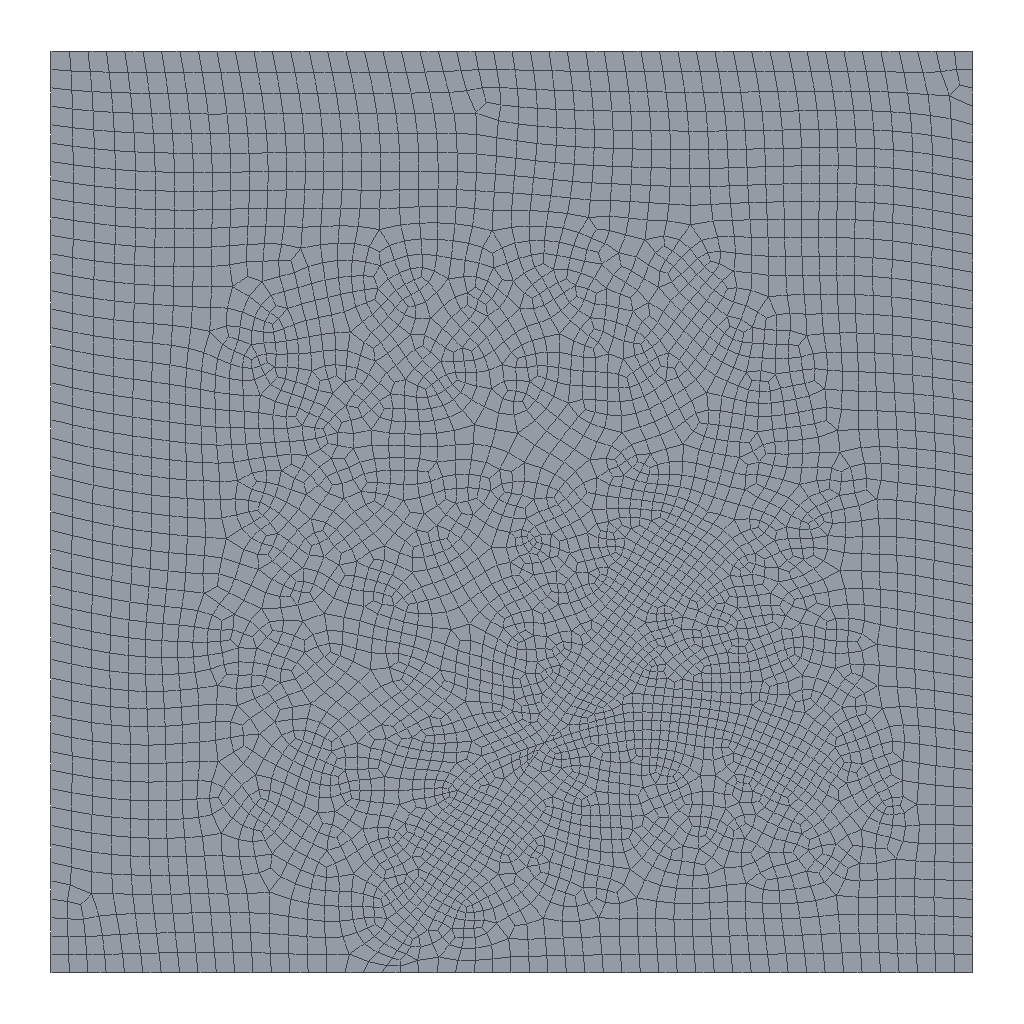Simulation study | abaqus
Set-up summary:
category,name,step,type,value,unit,region
solver,abaqus
solver,version,,,Abaqus/Standard 2020
units,not stated in the deck,,not stated
analysis,deck,,geostatic,geostatic
load_step,Step-1,Step-1,geostatic
load_step,Step-2,Step-2,soils
load_step,requested,,,2
mesh,nodes,,,4728
mesh,elements,,,4528
element_type,CPE4RP,,plane,4428
element_type,COH2D4P,,cohesive,100
load,load commands in deck,,count,1
bc,support commands in deck,,count,6
material,BASE,,in results
material,MATERIAL-2,,in results
check,setup vs results,,match,"per instance, exact: element labels, types and connectivity; labels of the nodes the elements use; coordinates of those nodes at SINGLE_PRECISION in 1 of 1 instance(s)"
Abaqus input file, long lists of numbers shortened:
*Heading
** Job name: Job-1 Model name: Model-1
** Generated by: Abaqus/CAE 2020
*Preprint, echo=NO, model=NO, history=NO, contact=NO
**
** PARTS
**
*Part, name=Part-1
*Node
      1,         100.,           0.
      2,           0.,           0.
** (4726 more lines like these left out)
*Element, type=CPE4RP
   1,    1,   10, 3981,  300
   2,  347,  394,  298,  299
** (4426 more lines like these left out)
*Element, type=COH2D4P
4429,    7,  187, 4530,    7,    7, 4592
4430,  187,  186, 4531, 4530, 4592, 4593
** (98 more lines like these left out)
*Nset, nset=Set-19
    1,    2,    3,    4,    5,    6,    7,    8,    9,   10,   11,   12,   13,   14,   15,   16
   17,   18,   19,   20,   21,   22,   23,   24,   25,   26,   27,   28,   29,   30,   31,   32
** (288 more lines like these left out)
*Elset, elset=Set-19, generate
    1,  4428,     1
*Elset, elset=CohesiveSeam-5-Elements, generate
 4429,  4490,     1
*Nset, nset=CohesiveSeam-5-TopNodes
    4,    5,    7,  125,  126,  127,  128,  129,  130,  131,  132,  133,  134,  135,  136,  137
  138,  139,  140,  141,  142,  143,  144,  145,  146,  147,  148,  149,  150,  151,  152,  153
** (2 more lines like these left out)
*Nset, nset=CohesiveSeam-5-BottomNodes
    7,  158,  159,  160,  161,  162,  163,  164,  165,  166,  167,  168,  169,  170,  171,  172
  173,  174,  175,  176,  177,  178,  179,  180,  181,  182,  183,  184,  185,  186,  187, 4561
** (2 more lines like these left out)
*Nset, nset=CohesiveSeam-5-MidNodes
    7, 4592, 4593, 4594, 4595, 4596, 4597, 4598, 4599, 4600, 4601, 4602, 4603, 4604, 4605, 4606
 4607, 4608, 4609, 4610, 4611, 4612, 4613, 4614, 4615, 4616, 4617, 4618, 4619, 4620, 4621, 4622
** (2 more lines like these left out)
*Elset, elset=CohesiveSeam-6-Elements, generate
 4491,  4528,     1
*Nset, nset=CohesiveSeam-6-TopNodes
    5,    6,    8,  155,  156,  157, 4659, 4660, 4661, 4662, 4663, 4664, 4665, 4666, 4667, 4668
 4669, 4670, 4671, 4672, 4673, 4674, 4675, 4676, 4677, 4678, 4679, 4680, 4681, 4682, 4683, 4684
** (1 more lines like these left out)
*Nset, nset=CohesiveSeam-6-BottomNodes
    6,    8,  188,  189,  190,  191,  192,  193,  194,  195,  196,  197,  198,  199,  200,  201
  202,  203,  204,  205,  206,  207,  208,  209,  210,  211,  212,  213,  214,  215,  216,  217
** (1 more lines like these left out)
*Nset, nset=CohesiveSeam-6-MidNodes
    6,    8, 4622, 4693, 4694, 4695, 4696, 4697, 4698, 4699, 4700, 4701, 4702, 4703, 4704, 4705
 4706, 4707, 4708, 4709, 4710, 4711, 4712, 4713, 4714, 4715, 4716, 4717, 4718, 4719, 4720, 4721
** (1 more lines like these left out)
*Nset, nset=inject
 4653,
*Elset, elset=initial-crack, generate
 4482,  4490,     1
*Nset, nset=plug1
 4621,
*Nset, nset=plug2
 4695,
*Elset, elset=__PickedSurf9_S1, internal
 1814, 1837, 1840, 1841, 1929, 1940, 2998, 3040, 3042, 3046, 3157, 4231, 4460, 4461, 4462, 4463
 4464, 4465, 4466, 4467, 4468, 4469, 4470, 4471, 4472, 4473, 4474, 4475, 4476, 4477, 4478, 4479
** (3 more lines like these left out)
*Elset, elset=__PickedSurf9_S4, internal
  359,  417,  449,  555, 1816, 1821, 1823, 1842, 2881, 3016, 3017, 3043, 3048, 3049, 3050, 3053
 3057, 3058, 3059, 3154
*Elset, elset=__PickedSurf9_S2, internal
  360,  416,  448,  484,  520,  554, 3037, 3039, 3045, 3055, 3060, 3125, 3131, 3144, 4232
*Elset, elset=__PickedSurf9_S3, internal
  362, 1791, 1825, 1839, 1878, 1892, 1893, 1894, 1902, 1928, 2914, 2937, 3038, 3044, 3047, 3051
 3052, 3056, 3141, 3149, 3158
*Surface, type=ELEMENT, name=_PickedSurf9, internal
__PickedSurf9_S1, S1
__PickedSurf9_S4, S4
__PickedSurf9_S2, S2
__PickedSurf9_S3, S3
*Elset, elset=__PickedSurf16_S1, internal, generate
 4460,  4490,     1
*Surface, type=ELEMENT, name=_PickedSurf16, internal
__PickedSurf16_S1, S1
*Elset, elset=__PickedSurf23_S4, internal
  359,  417,  449,  555, 1816, 1821, 1823, 1842, 2881, 3016, 3017, 3043, 3048, 3049, 3050, 3053
 3057, 3058, 3059, 3154
*Elset, elset=__PickedSurf23_S2, internal
  360,  416,  448,  484,  520,  554, 3037, 3039, 3045, 3055, 3060, 3125, 3131, 3144, 4232
*Elset, elset=__PickedSurf23_S3, internal
  362, 1791, 1825, 1839, 1878, 1892, 1893, 1894, 1902, 1928, 2914, 2937, 3038, 3044, 3047, 3051
 3052, 3056, 3141, 3149, 3158
*Elset, elset=__PickedSurf23_S1, internal
 1814, 1837, 1840, 1841, 1929, 1940, 2998, 3040, 3042, 3046, 3157, 4231, 4495, 4496, 4497, 4498
 4499, 4500, 4501, 4502, 4503, 4504, 4505, 4506, 4507, 4508, 4509, 4510, 4511, 4512, 4513, 4514
** (1 more lines like these left out)
*Surface, type=ELEMENT, name=_PickedSurf23, internal
__PickedSurf23_S4, S4
__PickedSurf23_S2, S2
__PickedSurf23_S3, S3
__PickedSurf23_S1, S1
*Elset, elset=__PickedSurf24_S4, internal
  359,  417,  449,  555, 1816, 1821, 1823, 1842, 2881, 3016, 3017, 3043, 3048, 3049, 3050, 3053
 3057, 3058, 3059, 3154
*Elset, elset=__PickedSurf24_S2, internal
  360,  416,  448,  484,  520,  554, 3037, 3039, 3045, 3055, 3060, 3125, 3131, 3144, 4232
*Elset, elset=__PickedSurf24_S3, internal
  362, 1791, 1825, 1839, 1878, 1892, 1893, 1894, 1902, 1928, 2914, 2937, 3038, 3044, 3047, 3051
 3052, 3056, 3141, 3149, 3158
*Elset, elset=__PickedSurf24_S1, internal
 1814, 1837, 1840, 1841, 1929, 1940, 2998, 3040, 3042, 3046, 3157, 4231, 4495, 4496, 4497, 4498
 4499, 4500, 4501, 4502, 4503, 4504, 4505, 4506, 4507, 4508, 4509, 4510, 4511, 4512, 4513, 4514
** (1 more lines like these left out)
*Surface, type=ELEMENT, name=_PickedSurf24, internal
__PickedSurf24_S4, S4
__PickedSurf24_S2, S2
__PickedSurf24_S3, S3
__PickedSurf24_S1, S1
*Elset, elset=__PickedSurf25_S4, internal
  359,  417,  449,  555, 1816, 1821, 1823, 1842, 2881, 3016, 3017, 3043, 3048, 3049, 3050, 3053
 3057, 3058, 3059, 3154
*Elset, elset=__PickedSurf25_S2, internal
  360,  416,  448,  484,  520,  554, 3037, 3039, 3045, 3055, 3060, 3125, 3131, 3144, 4232
*Elset, elset=__PickedSurf25_S3, internal
  362, 1791, 1825, 1839, 1878, 1892, 1893, 1894, 1902, 1928, 2914, 2937, 3038, 3044, 3047, 3051
 3052, 3056, 3141, 3149, 3158
*Elset, elset=__PickedSurf25_S1, internal
 1814, 1837, 1840, 1841, 1929, 1940, 2998, 3040, 3042, 3046, 3157, 4231, 4495, 4496, 4497, 4498
 4499, 4500, 4501, 4502, 4503, 4504, 4505, 4506, 4507, 4508, 4509, 4510, 4511, 4512, 4513, 4514
** (1 more lines like these left out)
*Surface, type=ELEMENT, name=_PickedSurf25, internal
__PickedSurf25_S4, S4
__PickedSurf25_S2, S2
__PickedSurf25_S3, S3
__PickedSurf25_S1, S1
*Elset, elset=__PickedSurf27_S1, internal
 1730, 1769, 1778, 1790, 1797, 1810, 1811, 1812, 2097, 2103, 2822, 3020, 3021, 3090, 3103, 3106
 3153, 4460, 4461, 4462, 4463, 4464, 4465, 4466, 4467, 4468, 4469, 4470, 4471, 4472, 4473, 4474
** (1 more lines like these left out)
*Elset, elset=__PickedSurf27_S3, internal
  577, 1728, 1788, 1798, 1804, 1808, 1818, 2102, 2104, 2106, 2821, 3017, 3033, 3099, 4429, 4430
 4431, 4432, 4433, 4434, 4435, 4436, 4437, 4438, 4439, 4440, 4441, 4442, 4443, 4444, 4445, 4446
** (1 more lines like these left out)
*Elset, elset=__PickedSurf27_S4, internal
  578,  690, 1729, 1745, 1765, 1785, 2067, 2083, 2660, 2710, 2720, 3022, 3026, 3029, 3032, 3035
 4230,
*Elset, elset=__PickedSurf27_S2, internal
 1727, 1746, 1780, 3019, 3024, 3027, 3028, 3031, 3034, 3076, 3083, 3084, 3097, 3111
*Surface, type=ELEMENT, name=_PickedSurf27, internal
__PickedSurf27_S1, S1
__PickedSurf27_S3, S3
__PickedSurf27_S4, S4
__PickedSurf27_S2, S2
*Elset, elset=__PickedSurf34_S1, internal
 1814, 1837, 1840, 1841, 1929, 1940, 2998, 3040, 3042, 3046, 3157, 4231, 4491, 4492, 4493, 4494
 4495, 4496, 4497, 4498, 4499, 4500, 4501, 4502, 4503, 4504, 4505, 4506, 4507, 4508, 4509, 4510
** (2 more lines like these left out)
*Elset, elset=__PickedSurf34_S4, internal
  359,  417,  449,  555, 1816, 1821, 1823, 1842, 2881, 3016, 3017, 3043, 3048, 3049, 3050, 3053
 3057, 3058, 3059, 3154
*Elset, elset=__PickedSurf34_S2, internal
  360,  416,  448,  484,  520,  554, 3037, 3039, 3045, 3055, 3060, 3125, 3131, 3144, 4232
*Elset, elset=__PickedSurf34_S3, internal
  362, 1791, 1825, 1839, 1878, 1892, 1893, 1894, 1902, 1928, 2914, 2937, 3038, 3044, 3047, 3051
 3052, 3056, 3141, 3149, 3158
*Surface, type=ELEMENT, name=_PickedSurf34, internal
__PickedSurf34_S1, S1
__PickedSurf34_S4, S4
__PickedSurf34_S2, S2
__PickedSurf34_S3, S3
*Elset, elset=__PickedSurf50_S1, internal
 1730, 1769, 1778, 1790, 1797, 1810, 1811, 1812, 2097, 2103, 2822, 3020, 3021, 3090, 3103, 3106
 3153, 4460, 4461, 4462, 4463, 4464, 4465, 4466, 4467, 4468, 4469, 4470, 4471, 4472, 4473, 4474
** (1 more lines like these left out)
*Elset, elset=__PickedSurf50_S3, internal
  577, 1728, 1788, 1798, 1804, 1808, 1818, 2102, 2104, 2106, 2821, 3017, 3033, 3099, 4429, 4430
 4431, 4432, 4433, 4434, 4435, 4436, 4437, 4438, 4439, 4440, 4441, 4442, 4443, 4444, 4445, 4446
** (1 more lines like these left out)
*Elset, elset=__PickedSurf50_S4, internal
  578,  690, 1729, 1745, 1765, 1785, 2067, 2083, 2660, 2710, 2720, 3022, 3026, 3029, 3032, 3035
 4230,
*Elset, elset=__PickedSurf50_S2, internal
 1727, 1746, 1780, 3019, 3024, 3027, 3028, 3031, 3034, 3076, 3083, 3084, 3097, 3111
*Surface, type=ELEMENT, name=_PickedSurf50, internal
__PickedSurf50_S1, S1
__PickedSurf50_S3, S3
__PickedSurf50_S4, S4
__PickedSurf50_S2, S2
*Elset, elset=__PickedSurf57_S1, internal
 1814, 1837, 1840, 1841, 1929, 1940, 2998, 3040, 3042, 3046, 3157, 4231, 4491, 4492, 4493, 4494
 4495, 4496, 4497, 4498, 4499, 4500, 4501, 4502, 4503, 4504, 4505, 4506, 4507, 4508, 4509, 4510
** (2 more lines like these left out)
*Elset, elset=__PickedSurf57_S4, internal
  359,  417,  449,  555, 1816, 1821, 1823, 1842, 2881, 3016, 3017, 3043, 3048, 3049, 3050, 3053
 3057, 3058, 3059, 3154
*Elset, elset=__PickedSurf57_S2, internal
  360,  416,  448,  484,  520,  554, 3037, 3039, 3045, 3055, 3060, 3125, 3131, 3144, 4232
*Elset, elset=__PickedSurf57_S3, internal
  362, 1791, 1825, 1839, 1878, 1892, 1893, 1894, 1902, 1928, 2914, 2937, 3038, 3044, 3047, 3051
 3052, 3056, 3141, 3149, 3158
*Surface, type=ELEMENT, name=_PickedSurf57, internal
__PickedSurf57_S1, S1
__PickedSurf57_S4, S4
__PickedSurf57_S2, S2
__PickedSurf57_S3, S3
*Elset, elset=_CohesiveSeam-5-TopSurf_S3, internal, generate
 4429,  4490,     1
*Surface, type=ELEMENT, name=CohesiveSeam-5-TopSurf
_CohesiveSeam-5-TopSurf_S3, S3
*Elset, elset=_CohesiveSeam-5-BottomSurf_S1, internal, generate
 4429,  4490,     1
*Surface, type=ELEMENT, name=CohesiveSeam-5-BottomSurf
_CohesiveSeam-5-BottomSurf_S1, S1
*Elset, elset=_CohesiveSeam-6-TopSurf_S3, internal, generate
 4491,  4528,     1
*Surface, type=ELEMENT, name=CohesiveSeam-6-TopSurf
_CohesiveSeam-6-TopSurf_S3, S3
*Elset, elset=_CohesiveSeam-6-BottomSurf_S1, internal, generate
 4491,  4528,     1
*Surface, type=ELEMENT, name=CohesiveSeam-6-BottomSurf
_CohesiveSeam-6-BottomSurf_S1, S1
** Section: base
*Solid Section, elset=Set-19, material=base
,
** Section: coh
*Cohesive Section, elset=CohesiveSeam-5-Elements, controls=EC-1, material=Material-2, response=TRACTION SEPARATION
,
** Section: coh
*Cohesive Section, elset=CohesiveSeam-6-Elements, controls=EC-1, material=Material-2, response=TRACTION SEPARATION
,
*Equation
2
4622, 8, 1
4658, 8, -1
*End Part
**
**
** ASSEMBLY
**
*Assembly, name=Assembly
**
*Instance, name=Part-1-1, part=Part-1
*End Instance
**
*Nset, nset=Set-1, instance=Part-1-1
    1,    2,    3,    4,    5,    6,    7,    8,    9,   10,   11,   12,   13,   14,   15,   16
   17,   18,   19,   20,   21,   22,   23,   24,   25,   26,   27,   28,   29,   30,   31,   32
** (288 more lines like these left out)
*Elset, elset=Set-1, instance=Part-1-1
    1,    2,    3,    4,    5,    6,    7,    8,    9,   10,   11,   12,   13,   14,   15,   16
   17,   18,   19,   20,   21,   22,   23,   24,   25,   26,   27,   28,   29,   30,   31,   32
** (279 more lines like these left out)
*Nset, nset=Set-2, instance=Part-1-1
    1,    2,    3,    4,    5,    6,    7,    8,    9,   10,   11,   12,   13,   14,   15,   16
   17,   18,   19,   20,   21,   22,   23,   24,   25,   26,   27,   28,   29,   30,   31,   32
** (288 more lines like these left out)
*Elset, elset=Set-2, instance=Part-1-1, generate
    1,  4428,     1
*Nset, nset=Set-3, instance=Part-1-1
   1,   2,   3,   9,  59,  60,  61,  62,  63,  64,  65,  66,  67,  68,  69,  70
  71,  72,  73,  74,  75,  76,  77,  78,  79,  80,  81,  82,  83,  84,  85,  86
** (5 more lines like these left out)
*Elset, elset=Set-3, instance=Part-1-1
    1,    2,    3,    4,    5,    6,    7,    8,    9,   10,   11,   12,   13,   14,   15,   16
   17,   18,   19,   20,   21,   22,   23,   24,   25,   26,   27,   28,   29,   30,   31,   32
** (5 more lines like these left out)
*Nset, nset=Set-4, instance=Part-1-1
    1,    2,    3,    4,    8,   10,   11,   12,   13,   14,   15,   16,   17,   18,   19,   20
   21,   22,   23,   24,   25,   26,   27,   28,   29,   30,   31,   32,   33,   34,   35,   36
** (7 more lines like these left out)
*Elset, elset=Set-4, instance=Part-1-1
    1,   49,   97,  145,  146,  193,  239,  284,  328,  359,  360,  362,  385,  416,  417,  418
  448,  449,  450,  484,  486,  520,  522,  554,  555,  556,  667,  692,  715,  740,  765,  788
** (9 more lines like these left out)
*End Assembly
**
** ELEMENT CONTROLS
**
*Section Controls, name=EC-1, ELEMENT DELETION=YES
1., 1., 1.
*Amplitude, name=Amp-1
             0.,              0.,             50.,              1.
**
** MATERIALS
**
*Material, name=Material-2
*Damage Initiation, criterion=MAXS
 1e+06, 5e+06, 5e+06
*Damage Evolution, type=DISPLACEMENT
 1e-09,
*Elastic, type=TRACTION
 1.5e+10, 1.5e+10, 1.5e+10
*Gap Flow
 0.001,
*Material, name=base
*Elastic
 1.5e+10, 0.25
*Permeability, specific=9800.
 1e-07, 0.2
**
** PREDEFINED FIELDS
**
** Name: Predefined Field-1   Type: Void ratio
*Initial Conditions, TYPE=RATIO
Set-1, 0.2
** Name: Predefined Field-2   Type: Stress
*Initial Conditions, type=STRESS
Set-2, -1e+06, -1e+06, -1e+06, 0.,
** ----------------------------------------------------------------
*initial conditions,type=initial gap
Part-1-1.initial-crack
**
** STEP: Step-1
**
*Step, name=Step-1, nlgeom=NO, unsymm=YES
*Geostatic
**
** BOUNDARY CONDITIONS
**
** Name: [REDACTED] : Displacement/rotation angle
*Boundary
Set-3, 1, 1
** Name: [REDACTED] : Displacement/rotation angle
*Boundary
Set-4, 2, 2
**
** OUTPUT REQUESTS
**
*Restart, write, frequency=0
**
** FIELD OUTPUT: F-Output-1
**
*Output, field, variable=PRESELECT
*Output, history, frequency=0
*End Step
** ----------------------------------------------------------------
**
** STEP: Step-2
**
*Step, name=Step-2, nlgeom=YES, unsymm=YES
*Soils, consolidation, end=PERIOD, utol=1e+25, creep=none
0.01, 500., 1e-05, 5.,
**
** BOUNDARY CONDITIONS
**
** Name: [REDACTED]
*Boundary
Part-1-1.plug1, 1, 1
Part-1-1.plug1, 2, 2
** Name: [REDACTED]
*Boundary
Part-1-1.plug2, 1, 1
Part-1-1.plug2, 2, 2
**
** LOADS
**
** Name: Load-inject Type: Concentrated [REDACTED] fluid
*Cflow, amplitude=Amp-1
Part-1-1.inject,  , -0.01
**
** OUTPUT REQUESTS
**
*Restart, write, frequency=0
**
** FIELD OUTPUT: F-Output-1
**
*Output, field
*Node Output
CF, PHILSM, POR, PSILSM, RF, U
*Element Output, directions=YES
E, FLUVR, FLVEL, LE, MISES, S, SAT, SDEG, VOIDR,pfopen
*Contact Output
CSDMG, PFL, PFLA, PTL, PTLA
**
** HISTORY OUTPUT: H-Output-1
**
*Output, history
*Node Output, nset=Part-1-1.inject
POR,
*End Step
Results summary:
result,step,,completed,increments=1 time=1.0/1.0
result,step,,partial,increments=100 time=313.859/500.0
result,analysis,,,"soils, consolidation"
result,last_loadstep,,,2
result,primary field,,,"U, POR"
result,reaction total,,FX,474016222.0,model units
result,reaction total,,FY,-247760883.875,model units
result,reaction total,,FZ,0.0,model units